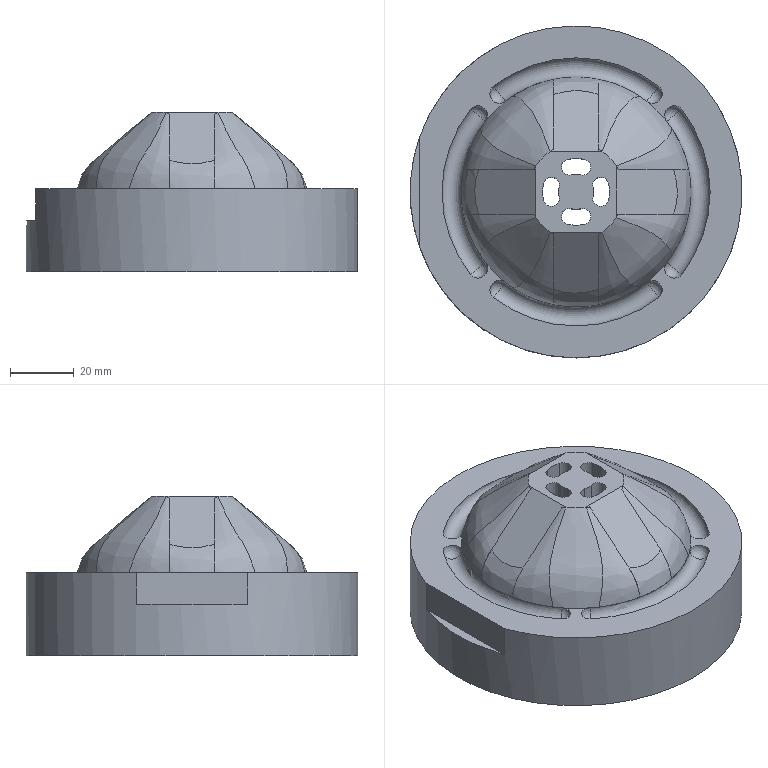NC program | NX | posted with a generic post | part box 104 x 104 x 49.86 mm
Lines 2861 to 4138 of 41131:
(PLANAR_MILL , TOOL : B)
N5714 M6
N5716 G54
N5718 G17 G0 G90 X-10.762 Y37.49 S2122 M3
N5720 G43 Z20. H0
N5722 Z-23.86
N5724 G94 G1 X-12.845 Y36.834 Z-23.87 F785.
N5726 X-15.067 Y35.983 Z-23.88
N5728 X-17.233 Y34.997 Z-23.891
N5730 X-19.335 Y33.881 Z-23.901
N5732 X-21.365 Y32.64 Z-23.911
N5734 X-23.315 Y31.276 Z-23.922
N5736 X-24.011 Y30.732 Z-23.926
N5738 X-23.315 Y31.276 Z-23.929
N5740 X-21.365 Y32.64 Z-23.94
N5742 X-19.335 Y33.881 Z-23.95
N5744 X-17.233 Y34.997 Z-23.961
N5746 X-15.067 Y35.983 Z-23.971
N5748 X-12.845 Y36.834 Z-23.981
N5750 X-10.576 Y37.549 Z-23.992
N5752 X-8.267 Y38.124 Z-24.002
N5754 X-5.927 Y38.557 Z-24.013
N5756 X-3.565 Y38.847 Z-24.023
N5758 X-1.19 Y38.992 Z-24.033
N5760 X1.19 Z-24.044
N5762 X3.565 Y38.847 Z-24.054
N5764 X5.927 Y38.557 Z-24.064
N5766 X8.267 Y38.124 Z-24.075
N5768 X10.576 Y37.549 Z-24.085
N5770 X12.845 Y36.834 Z-24.096
N5772 X15.067 Y35.983 Z-24.106
N5774 X17.233 Y34.997 Z-24.116
N5776 X19.335 Y33.881 Z-24.127
N5778 X21.365 Y32.64 Z-24.137
N5780 X23.315 Y31.276 Z-24.147
N5782 X24.011 Y30.732 Z-24.151
N5784 X23.315 Y31.276 Z-24.155
N5786 X21.365 Y32.64 Z-24.166
N5788 X19.335 Y33.881 Z-24.176
N5790 X17.233 Y34.997 Z-24.186
N5792 X15.067 Y35.983 Z-24.197
N5794 X12.845 Y36.834 Z-24.207
N5796 X10.576 Y37.549 Z-24.217
N5798 X8.267 Y38.124 Z-24.228
N5800 X5.927 Y38.557 Z-24.238
N5802 X3.565 Y38.847 Z-24.249
N5804 X1.19 Y38.992 Z-24.259
N5806 X-1.19 Z-24.269
N5808 X-3.565 Y38.847 Z-24.28
N5810 X-5.927 Y38.557 Z-24.29
N5812 X-8.267 Y38.124 Z-24.301
N5814 X-10.576 Y37.549 Z-24.311
N5816 X-12.845 Y36.834 Z-24.321
N5818 X-15.067 Y35.983 Z-24.332
N5820 X-17.233 Y34.997 Z-24.342
N5822 X-19.335 Y33.881 Z-24.352
N5824 X-21.365 Y32.64 Z-24.363
N5826 X-23.315 Y31.276 Z-24.373
N5828 X-24.011 Y30.732 Z-24.377
N5830 X-23.315 Y31.276 Z-24.381
N5832 X-21.365 Y32.64 Z-24.391
N5834 X-19.335 Y33.881 Z-24.402
N5836 X-17.233 Y34.997 Z-24.412
N5838 X-15.067 Y35.983 Z-24.422
N5840 X-12.845 Y36.834 Z-24.433
N5842 X-10.576 Y37.549 Z-24.443
N5844 X-8.267 Y38.124 Z-24.454
N5846 X-5.927 Y38.557 Z-24.464
N5848 X-3.565 Y38.847 Z-24.474
N5850 X-1.19 Y38.992 Z-24.485
N5852 X1.19 Z-24.495
N5854 X3.565 Y38.847 Z-24.506
N5856 X5.927 Y38.557 Z-24.516
N5858 X8.267 Y38.124 Z-24.526
N5860 X10.576 Y37.549 Z-24.537
N5862 X12.845 Y36.834 Z-24.547
N5864 X15.067 Y35.983 Z-24.557
N5866 X17.233 Y34.997 Z-24.568
N5868 X19.335 Y33.881 Z-24.578
N5870 X21.365 Y32.64 Z-24.589
N5872 X23.315 Y31.276 Z-24.599
N5874 X24.011 Y30.732 Z-24.603
N5876 X23.315 Y31.276 Z-24.607
N5878 X21.365 Y32.64 Z-24.617
N5880 X19.335 Y33.881 Z-24.627
N5882 X17.233 Y34.997 Z-24.638
N5884 X15.067 Y35.983 Z-24.648
N5886 X12.845 Y36.834 Z-24.659
N5888 X10.576 Y37.549 Z-24.669
N5890 X8.267 Y38.124 Z-24.679
N5892 X5.927 Y38.557 Z-24.69
N5894 X3.565 Y38.847 Z-24.7
N5896 X1.19 Y38.992 Z-24.711
N5898 X-1.19 Z-24.721
N5900 X-3.565 Y38.847 Z-24.731
N5902 X-5.927 Y38.557 Z-24.742
N5904 X-8.267 Y38.124 Z-24.752
N5906 X-10.576 Y37.549 Z-24.762
N5908 X-12.845 Y36.834 Z-24.773
N5910 X-15.067 Y35.983 Z-24.783
N5912 X-17.233 Y34.997 Z-24.794
N5914 X-19.335 Y33.881 Z-24.804
N5916 X-21.365 Y32.64 Z-24.814
N5918 X-23.315 Y31.276 Z-24.825
N5920 X-24.011 Y30.732 Z-24.829
N5922 X-23.315 Y31.276 Z-24.832
N5924 X-21.365 Y32.64 Z-24.843
N5926 X-19.335 Y33.881 Z-24.853
N5928 X-17.233 Y34.997 Z-24.864
N5930 X-15.067 Y35.983 Z-24.874
N5932 X-12.845 Y36.834 Z-24.884
N5934 X-10.576 Y37.549 Z-24.895
N5936 X-8.267 Y38.124 Z-24.905
N5938 X-5.927 Y38.557 Z-24.915
N5940 X-3.565 Y38.847 Z-24.926
N5942 X-1.19 Y38.992 Z-24.936
N5944 X1.19 Z-24.947
N5946 X3.565 Y38.847 Z-24.957
N5948 X5.927 Y38.557 Z-24.967
N5950 X8.267 Y38.124 Z-24.978
N5952 X10.576 Y37.549 Z-24.988
N5954 X12.845 Y36.834 Z-24.999
N5956 X15.067 Y35.983 Z-25.009
N5958 X17.233 Y34.997 Z-25.019
N5960 X19.335 Y33.881 Z-25.03
N5962 X21.365 Y32.64 Z-25.04
N5964 X23.315 Y31.276 Z-25.05
N5966 X24.011 Y30.732 Z-25.054
N5968 X23.315 Y31.276 Z-25.058
N5970 X21.365 Y32.64 Z-25.069
N5972 X19.335 Y33.881 Z-25.079
N5974 X17.233 Y34.997 Z-25.089
N5976 X15.067 Y35.983 Z-25.1
N5978 X12.845 Y36.834 Z-25.11
N5980 X10.576 Y37.549 Z-25.12
N5982 X8.267 Y38.124 Z-25.131
N5984 X5.927 Y38.557 Z-25.141
N5986 X3.565 Y38.847 Z-25.152
N5988 X1.19 Y38.992 Z-25.162
N5990 X-1.19 Z-25.172
N5992 X-3.565 Y38.847 Z-25.183
N5994 X-5.927 Y38.557 Z-25.193
N5996 X-8.267 Y38.124 Z-25.204
N5998 X-10.576 Y37.549 Z-25.214
N6000 X-12.845 Y36.834 Z-25.224
N6002 X-15.067 Y35.983 Z-25.235
N6004 X-17.233 Y34.997 Z-25.245
N6006 X-19.335 Y33.881 Z-25.255
N6008 X-21.365 Y32.64 Z-25.266
N6010 X-23.315 Y31.276 Z-25.276
N6012 X-24.011 Y30.732 Z-25.28
N6014 X-23.315 Y31.276 Z-25.284
N6016 X-21.365 Y32.64 Z-25.294
N6018 X-19.335 Y33.881 Z-25.305
N6020 X-17.233 Y34.997 Z-25.315
N6022 X-15.067 Y35.983 Z-25.325
N6024 X-12.845 Y36.834 Z-25.336
N6026 X-10.576 Y37.549 Z-25.346
N6028 X-8.267 Y38.124 Z-25.357
N6030 X-5.927 Y38.557 Z-25.367
N6032 X-3.565 Y38.847 Z-25.377
N6034 X-1.19 Y38.992 Z-25.388
N6036 X1.19 Z-25.398
N6038 X3.565 Y38.847 Z-25.409
N6040 X5.927 Y38.557 Z-25.419
N6042 X8.267 Y38.124 Z-25.429
N6044 X10.576 Y37.549 Z-25.44
N6046 X12.845 Y36.834 Z-25.45
N6048 X15.067 Y35.983 Z-25.46
N6050 X17.233 Y34.997 Z-25.471
N6052 X19.335 Y33.881 Z-25.481
N6054 X21.365 Y32.64 Z-25.492
N6056 X23.315 Y31.276 Z-25.502
N6058 X24.011 Y30.732 Z-25.506
N6060 X23.315 Y31.276 Z-25.51
N6062 X21.365 Y32.64 Z-25.52
N6064 X19.335 Y33.881 Z-25.53
N6066 X17.233 Y34.997 Z-25.541
N6068 X15.067 Y35.983 Z-25.551
N6070 X12.845 Y36.834 Z-25.562
N6072 X10.576 Y37.549 Z-25.572
N6074 X8.267 Y38.124 Z-25.582
N6076 X5.927 Y38.557 Z-25.593
N6078 X3.565 Y38.847 Z-25.603
N6080 X1.19 Y38.992 Z-25.614
N6082 X-1.19 Z-25.624
N6084 X-3.565 Y38.847 Z-25.634
N6086 X-5.927 Y38.557 Z-25.645
N6088 X-8.267 Y38.124 Z-25.655
N6090 X-10.576 Y37.549 Z-25.665
N6092 X-12.845 Y36.834 Z-25.676
N6094 X-15.067 Y35.983 Z-25.686
N6096 X-17.233 Y34.997 Z-25.697
N6098 X-19.335 Y33.881 Z-25.707
N6100 X-21.365 Y32.64 Z-25.717
N6102 X-23.315 Y31.276 Z-25.728
N6104 X-24.011 Y30.732 Z-25.732
N6106 X-23.315 Y31.276 Z-25.735
N6108 X-21.365 Y32.64 Z-25.746
N6110 X-19.335 Y33.881 Z-25.756
N6112 X-17.233 Y34.997 Z-25.767
N6114 X-15.067 Y35.983 Z-25.777
N6116 X-12.845 Y36.834 Z-25.787
N6118 X-10.576 Y37.549 Z-25.798
N6120 X-8.267 Y38.124 Z-25.808
N6122 X-5.927 Y38.557 Z-25.818
N6124 X-3.565 Y38.847 Z-25.829
N6126 X-1.19 Y38.992 Z-25.839
N6128 X1.19 Z-25.85
N6130 X3.565 Y38.847 Z-25.86
N6132 X5.927 Y38.557 Z-25.87
N6134 X8.267 Y38.124 Z-25.881
N6136 X10.576 Y37.549 Z-25.891
N6138 X12.845 Y36.834 Z-25.902
N6140 X15.067 Y35.983 Z-25.912
N6142 X17.233 Y34.997 Z-25.922
N6144 X19.335 Y33.881 Z-25.933
N6146 X21.365 Y32.64 Z-25.943
N6148 X23.315 Y31.276 Z-25.953
N6150 X24.011 Y30.732 Z-25.957
N6152 X23.315 Y31.276 Z-25.961
N6154 X21.365 Y32.64 Z-25.972
N6156 X19.335 Y33.881 Z-25.982
N6158 X17.233 Y34.997 Z-25.992
N6160 X15.067 Y35.983 Z-26.003
N6162 X12.845 Y36.834 Z-26.013
N6164 X10.576 Y37.549 Z-26.023
N6166 X8.267 Y38.124 Z-26.034
N6168 X5.927 Y38.557 Z-26.044
N6170 X3.565 Y38.847 Z-26.055
N6172 X1.19 Y38.992 Z-26.065
N6174 X-1.19 Z-26.075
N6176 X-3.565 Y38.847 Z-26.086
N6178 X-5.927 Y38.557 Z-26.096
N6180 X-8.267 Y38.124 Z-26.107
N6182 X-10.576 Y37.549 Z-26.117
N6184 X-12.845 Y36.834 Z-26.127
N6186 X-15.067 Y35.983 Z-26.138
N6188 X-17.233 Y34.997 Z-26.148
N6190 X-19.335 Y33.881 Z-26.158
N6192 X-21.365 Y32.64 Z-26.169
N6194 X-23.315 Y31.276 Z-26.179
N6196 X-24.011 Y30.732 Z-26.183
N6198 X-23.315 Y31.276 Z-26.187
N6200 X-21.365 Y32.64 Z-26.197
N6202 X-19.335 Y33.881 Z-26.208
N6204 X-17.233 Y34.997 Z-26.218
N6206 X-15.067 Y35.983 Z-26.228
N6208 X-12.845 Y36.834 Z-26.239
N6210 X-10.576 Y37.549 Z-26.249
N6212 X-8.267 Y38.124 Z-26.26
N6214 X-5.927 Y38.557 Z-26.27
N6216 X-3.565 Y38.847 Z-26.28
N6218 X-1.19 Y38.992 Z-26.291
N6220 X1.19 Z-26.301
N6222 X3.565 Y38.847 Z-26.312
N6224 X5.927 Y38.557 Z-26.322
N6226 X8.267 Y38.124 Z-26.332
N6228 X10.576 Y37.549 Z-26.343
N6230 X12.845 Y36.834 Z-26.353
N6232 X15.067 Y35.983 Z-26.363
N6234 X17.233 Y34.997 Z-26.374
N6236 X19.335 Y33.881 Z-26.384
N6238 X21.365 Y32.64 Z-26.395
N6240 X23.315 Y31.276 Z-26.405
N6242 X24.011 Y30.732 Z-26.409
N6244 X23.315 Y31.276 Z-26.413
N6246 X21.365 Y32.64 Z-26.423
N6248 X19.335 Y33.881 Z-26.433
N6250 X17.233 Y34.997 Z-26.444
N6252 X15.067 Y35.983 Z-26.454
N6254 X12.845 Y36.834 Z-26.465
N6256 X10.576 Y37.549 Z-26.475
N6258 X8.267 Y38.124 Z-26.485
N6260 X5.927 Y38.557 Z-26.496
N6262 X3.565 Y38.847 Z-26.506
N6264 X1.19 Y38.992 Z-26.516
N6266 X-1.19 Z-26.527
N6268 X-3.565 Y38.847 Z-26.537
N6270 X-5.927 Y38.557 Z-26.548
N6272 X-8.267 Y38.124 Z-26.558
N6274 X-10.576 Y37.549 Z-26.568
N6276 X-12.845 Y36.834 Z-26.579
N6278 X-15.067 Y35.983 Z-26.589
N6280 X-17.233 Y34.997 Z-26.6
N6282 X-19.335 Y33.881 Z-26.61
N6284 X-21.365 Y32.64 Z-26.62
N6286 X-23.315 Y31.276 Z-26.631
N6288 X-24.011 Y30.732 Z-26.635
N6290 X-23.315 Y31.276 Z-26.638
N6292 X-21.365 Y32.64 Z-26.649
N6294 X-19.335 Y33.881 Z-26.659
N6296 X-17.233 Y34.997 Z-26.67
N6298 X-15.067 Y35.983 Z-26.68
N6300 X-12.845 Y36.834 Z-26.69
N6302 X-10.576 Y37.549 Z-26.701
N6304 X-8.267 Y38.124 Z-26.711
N6306 X-5.927 Y38.557 Z-26.721
N6308 X-3.565 Y38.847 Z-26.732
N6310 X-1.19 Y38.992 Z-26.742
N6312 X1.19 Z-26.753
N6314 X3.565 Y38.847 Z-26.763
N6316 X5.927 Y38.557 Z-26.773
N6318 X8.267 Y38.124 Z-26.784
N6320 X10.576 Y37.549 Z-26.794
N6322 X12.845 Y36.834 Z-26.805
N6324 X15.067 Y35.983 Z-26.815
N6326 X17.233 Y34.997 Z-26.825
N6328 X19.335 Y33.881 Z-26.836
N6330 X21.365 Y32.64 Z-26.846
N6332 X23.315 Y31.276 Z-26.856
N6334 X24.011 Y30.732 Z-26.86
N6336 G3 X-24.011 Y30.732 R39.
N6338 G1 Z-23.86
N6340 G0 Z20.
N6342 X-37.49 Y-10.762
N6344 Z-23.86
N6346 G1 X-36.834 Y-12.845 Z-23.87
N6348 X-35.983 Y-15.067 Z-23.88
N6350 X-34.997 Y-17.233 Z-23.891
N6352 X-33.881 Y-19.335 Z-23.901
N6354 X-32.64 Y-21.365 Z-23.911
N6356 X-31.276 Y-23.315 Z-23.922
N6358 X-30.732 Y-24.011 Z-23.926
N6360 X-31.276 Y-23.315 Z-23.929
N6362 X-32.64 Y-21.365 Z-23.94
N6364 X-33.881 Y-19.335 Z-23.95
N6366 X-34.997 Y-17.233 Z-23.961
N6368 X-35.983 Y-15.067 Z-23.971
N6370 X-36.834 Y-12.845 Z-23.981
N6372 X-37.549 Y-10.576 Z-23.992
N6374 X-38.124 Y-8.267 Z-24.002
N6376 X-38.557 Y-5.927 Z-24.013
N6378 X-38.847 Y-3.565 Z-24.023
N6380 X-38.992 Y-1.19 Z-24.033
N6382 Y1.19 Z-24.044
N6384 X-38.847 Y3.565 Z-24.054
N6386 X-38.557 Y5.927 Z-24.064
N6388 X-38.124 Y8.267 Z-24.075
N6390 X-37.549 Y10.576 Z-24.085
N6392 X-36.834 Y12.845 Z-24.096
N6394 X-35.983 Y15.067 Z-24.106
N6396 X-34.997 Y17.233 Z-24.116
N6398 X-33.881 Y19.335 Z-24.127
N6400 X-32.64 Y21.365 Z-24.137
N6402 X-31.276 Y23.315 Z-24.147
N6404 X-30.732 Y24.011 Z-24.151
N6406 X-31.276 Y23.315 Z-24.155
N6408 X-32.64 Y21.365 Z-24.166
N6410 X-33.881 Y19.335 Z-24.176
N6412 X-34.997 Y17.233 Z-24.186
N6414 X-35.983 Y15.067 Z-24.197
N6416 X-36.834 Y12.845 Z-24.207
N6418 X-37.549 Y10.576 Z-24.217
N6420 X-38.124 Y8.267 Z-24.228
N6422 X-38.557 Y5.927 Z-24.238
N6424 X-38.847 Y3.565 Z-24.249
N6426 X-38.992 Y1.19 Z-24.259
N6428 Y-1.19 Z-24.269
N6430 X-38.847 Y-3.565 Z-24.28
N6432 X-38.557 Y-5.927 Z-24.29
N6434 X-38.124 Y-8.267 Z-24.301
N6436 X-37.549 Y-10.576 Z-24.311
N6438 X-36.834 Y-12.845 Z-24.321
N6440 X-35.983 Y-15.067 Z-24.332
N6442 X-34.997 Y-17.233 Z-24.342
N6444 X-33.881 Y-19.335 Z-24.352
N6446 X-32.64 Y-21.365 Z-24.363
N6448 X-31.276 Y-23.315 Z-24.373
N6450 X-30.732 Y-24.011 Z-24.377
N6452 X-31.276 Y-23.315 Z-24.381
N6454 X-32.64 Y-21.365 Z-24.391
N6456 X-33.881 Y-19.335 Z-24.402
N6458 X-34.997 Y-17.233 Z-24.412
N6460 X-35.983 Y-15.067 Z-24.422
N6462 X-36.834 Y-12.845 Z-24.433
N6464 X-37.549 Y-10.576 Z-24.443
N6466 X-38.124 Y-8.267 Z-24.454
N6468 X-38.557 Y-5.927 Z-24.464
N6470 X-38.847 Y-3.565 Z-24.474
N6472 X-38.992 Y-1.19 Z-24.485
N6474 Y1.19 Z-24.495
N6476 X-38.847 Y3.565 Z-24.506
N6478 X-38.557 Y5.927 Z-24.516
N6480 X-38.124 Y8.267 Z-24.526
N6482 X-37.549 Y10.576 Z-24.537
N6484 X-36.834 Y12.845 Z-24.547
N6486 X-35.983 Y15.067 Z-24.557
N6488 X-34.997 Y17.233 Z-24.568
N6490 X-33.881 Y19.335 Z-24.578
N6492 X-32.64 Y21.365 Z-24.589
N6494 X-31.276 Y23.315 Z-24.599
N6496 X-30.732 Y24.011 Z-24.603
N6498 X-31.276 Y23.315 Z-24.607
N6500 X-32.64 Y21.365 Z-24.617
N6502 X-33.881 Y19.335 Z-24.627
N6504 X-34.997 Y17.233 Z-24.638
N6506 X-35.983 Y15.067 Z-24.648
N6508 X-36.834 Y12.845 Z-24.659
N6510 X-37.549 Y10.576 Z-24.669
N6512 X-38.124 Y8.267 Z-24.679
N6514 X-38.557 Y5.927 Z-24.69
N6516 X-38.847 Y3.565 Z-24.7
N6518 X-38.992 Y1.19 Z-24.711
N6520 Y-1.19 Z-24.721
N6522 X-38.847 Y-3.565 Z-24.731
N6524 X-38.557 Y-5.927 Z-24.742
N6526 X-38.124 Y-8.267 Z-24.752
N6528 X-37.549 Y-10.576 Z-24.762
N6530 X-36.834 Y-12.845 Z-24.773
N6532 X-35.983 Y-15.067 Z-24.783
N6534 X-34.997 Y-17.233 Z-24.794
N6536 X-33.881 Y-19.335 Z-24.804
N6538 X-32.64 Y-21.365 Z-24.814
N6540 X-31.276 Y-23.315 Z-24.825
N6542 X-30.732 Y-24.011 Z-24.829
N6544 X-31.276 Y-23.315 Z-24.832
N6546 X-32.64 Y-21.365 Z-24.843
N6548 X-33.881 Y-19.335 Z-24.853
N6550 X-34.997 Y-17.233 Z-24.864
N6552 X-35.983 Y-15.067 Z-24.874
N6554 X-36.834 Y-12.845 Z-24.884
N6556 X-37.549 Y-10.576 Z-24.895
N6558 X-38.124 Y-8.267 Z-24.905
N6560 X-38.557 Y-5.927 Z-24.915
N6562 X-38.847 Y-3.565 Z-24.926
N6564 X-38.992 Y-1.19 Z-24.936
N6566 Y1.19 Z-24.947
N6568 X-38.847 Y3.565 Z-24.957
N6570 X-38.557 Y5.927 Z-24.967
N6572 X-38.124 Y8.267 Z-24.978
N6574 X-37.549 Y10.576 Z-24.988
N6576 X-36.834 Y12.845 Z-24.999
N6578 X-35.983 Y15.067 Z-25.009
N6580 X-34.997 Y17.233 Z-25.019
N6582 X-33.881 Y19.335 Z-25.03
N6584 X-32.64 Y21.365 Z-25.04
N6586 X-31.276 Y23.315 Z-25.05
N6588 X-30.732 Y24.011 Z-25.054
N6590 X-31.276 Y23.315 Z-25.058
N6592 X-32.64 Y21.365 Z-25.069
N6594 X-33.881 Y19.335 Z-25.079
N6596 X-34.997 Y17.233 Z-25.089
N6598 X-35.983 Y15.067 Z-25.1
N6600 X-36.834 Y12.845 Z-25.11
N6602 X-37.549 Y10.576 Z-25.12
N6604 X-38.124 Y8.267 Z-25.131
N6606 X-38.557 Y5.927 Z-25.141
N6608 X-38.847 Y3.565 Z-25.152
N6610 X-38.992 Y1.19 Z-25.162
N6612 Y-1.19 Z-25.172
N6614 X-38.847 Y-3.565 Z-25.183
N6616 X-38.557 Y-5.927 Z-25.193
N6618 X-38.124 Y-8.267 Z-25.204
N6620 X-37.549 Y-10.576 Z-25.214
N6622 X-36.834 Y-12.845 Z-25.224
N6624 X-35.983 Y-15.067 Z-25.235
N6626 X-34.997 Y-17.233 Z-25.245
N6628 X-33.881 Y-19.335 Z-25.255
N6630 X-32.64 Y-21.365 Z-25.266
N6632 X-31.276 Y-23.315 Z-25.276
N6634 X-30.732 Y-24.011 Z-25.28
N6636 X-31.276 Y-23.315 Z-25.284
N6638 X-32.64 Y-21.365 Z-25.294
N6640 X-33.881 Y-19.335 Z-25.305
N6642 X-34.997 Y-17.233 Z-25.315
N6644 X-35.983 Y-15.067 Z-25.325
N6646 X-36.834 Y-12.845 Z-25.336
N6648 X-37.549 Y-10.576 Z-25.346
N6650 X-38.124 Y-8.267 Z-25.357
N6652 X-38.557 Y-5.927 Z-25.367
N6654 X-38.847 Y-3.565 Z-25.377
N6656 X-38.992 Y-1.19 Z-25.388
N6658 Y1.19 Z-25.398
N6660 X-38.847 Y3.565 Z-25.409
N6662 X-38.557 Y5.927 Z-25.419
N6664 X-38.124 Y8.267 Z-25.429
N6666 X-37.549 Y10.576 Z-25.44
N6668 X-36.834 Y12.845 Z-25.45
N6670 X-35.983 Y15.067 Z-25.46
N6672 X-34.997 Y17.233 Z-25.471
N6674 X-33.881 Y19.335 Z-25.481
N6676 X-32.64 Y21.365 Z-25.492
N6678 X-31.276 Y23.315 Z-25.502
N6680 X-30.732 Y24.011 Z-25.506
N6682 X-31.276 Y23.315 Z-25.51
N6684 X-32.64 Y21.365 Z-25.52
N6686 X-33.881 Y19.335 Z-25.53
N6688 X-34.997 Y17.233 Z-25.541
N6690 X-35.983 Y15.067 Z-25.551
N6692 X-36.834 Y12.845 Z-25.562
N6694 X-37.549 Y10.576 Z-25.572
N6696 X-38.124 Y8.267 Z-25.582
N6698 X-38.557 Y5.927 Z-25.593
N6700 X-38.847 Y3.565 Z-25.603
N6702 X-38.992 Y1.19 Z-25.614
N6704 Y-1.19 Z-25.624
N6706 X-38.847 Y-3.565 Z-25.634
N6708 X-38.557 Y-5.927 Z-25.645
N6710 X-38.124 Y-8.267 Z-25.655
N6712 X-37.549 Y-10.576 Z-25.665
N6714 X-36.834 Y-12.845 Z-25.676
N6716 X-35.983 Y-15.067 Z-25.686
N6718 X-34.997 Y-17.233 Z-25.697
N6720 X-33.881 Y-19.335 Z-25.707
N6722 X-32.64 Y-21.365 Z-25.717
N6724 X-31.276 Y-23.315 Z-25.728
N6726 X-30.732 Y-24.011 Z-25.732
N6728 X-31.276 Y-23.315 Z-25.735
N6730 X-32.64 Y-21.365 Z-25.746
N6732 X-33.881 Y-19.335 Z-25.756
N6734 X-34.997 Y-17.233 Z-25.767
N6736 X-35.983 Y-15.067 Z-25.777
N6738 X-36.834 Y-12.845 Z-25.787
N6740 X-37.549 Y-10.576 Z-25.798
N6742 X-38.124 Y-8.267 Z-25.808
N6744 X-38.557 Y-5.927 Z-25.818
N6746 X-38.847 Y-3.565 Z-25.829
N6748 X-38.992 Y-1.19 Z-25.839
N6750 Y1.19 Z-25.85
N6752 X-38.847 Y3.565 Z-25.86
N6754 X-38.557 Y5.927 Z-25.87
N6756 X-38.124 Y8.267 Z-25.881
N6758 X-37.549 Y10.576 Z-25.891
N6760 X-36.834 Y12.845 Z-25.902
N6762 X-35.983 Y15.067 Z-25.912
N6764 X-34.997 Y17.233 Z-25.922
N6766 X-33.881 Y19.335 Z-25.933
N6768 X-32.64 Y21.365 Z-25.943
N6770 X-31.276 Y23.315 Z-25.953
N6772 X-30.732 Y24.011 Z-25.957
N6774 X-31.276 Y23.315 Z-25.961
N6776 X-32.64 Y21.365 Z-25.972
N6778 X-33.881 Y19.335 Z-25.982
N6780 X-34.997 Y17.233 Z-25.992
N6782 X-35.983 Y15.067 Z-26.003
N6784 X-36.834 Y12.845 Z-26.013
N6786 X-37.549 Y10.576 Z-26.023
N6788 X-38.124 Y8.267 Z-26.034
N6790 X-38.557 Y5.927 Z-26.044
N6792 X-38.847 Y3.565 Z-26.055
N6794 X-38.992 Y1.19 Z-26.065
N6796 Y-1.19 Z-26.075
N6798 X-38.847 Y-3.565 Z-26.086
N6800 X-38.557 Y-5.927 Z-26.096
N6802 X-38.124 Y-8.267 Z-26.107
N6804 X-37.549 Y-10.576 Z-26.117
N6806 X-36.834 Y-12.845 Z-26.127
N6808 X-35.983 Y-15.067 Z-26.138
N6810 X-34.997 Y-17.233 Z-26.148
N6812 X-33.881 Y-19.335 Z-26.158
N6814 X-32.64 Y-21.365 Z-26.169
N6816 X-31.276 Y-23.315 Z-26.179
N6818 X-30.732 Y-24.011 Z-26.183
N6820 X-31.276 Y-23.315 Z-26.187
N6822 X-32.64 Y-21.365 Z-26.197
N6824 X-33.881 Y-19.335 Z-26.208
N6826 X-34.997 Y-17.233 Z-26.218
N6828 X-35.983 Y-15.067 Z-26.228
N6830 X-36.834 Y-12.845 Z-26.239
N6832 X-37.549 Y-10.576 Z-26.249
N6834 X-38.124 Y-8.267 Z-26.26
N6836 X-38.557 Y-5.927 Z-26.27
N6838 X-38.847 Y-3.565 Z-26.28
N6840 X-38.992 Y-1.19 Z-26.291
N6842 Y1.19 Z-26.301
N6844 X-38.847 Y3.565 Z-26.312
N6846 X-38.557 Y5.927 Z-26.322
N6848 X-38.124 Y8.267 Z-26.332
N6850 X-37.549 Y10.576 Z-26.343
N6852 X-36.834 Y12.845 Z-26.353
N6854 X-35.983 Y15.067 Z-26.363
N6856 X-34.997 Y17.233 Z-26.374
N6858 X-33.881 Y19.335 Z-26.384
N6860 X-32.64 Y21.365 Z-26.395
N6862 X-31.276 Y23.315 Z-26.405
N6864 X-30.732 Y24.011 Z-26.409
N6866 X-31.276 Y23.315 Z-26.413
N6868 X-32.64 Y21.365 Z-26.423
N6870 X-33.881 Y19.335 Z-26.433
N6872 X-34.997 Y17.233 Z-26.444
N6874 X-35.983 Y15.067 Z-26.454
N6876 X-36.834 Y12.845 Z-26.465
N6878 X-37.549 Y10.576 Z-26.475
N6880 X-38.124 Y8.267 Z-26.485
N6882 X-38.557 Y5.927 Z-26.496
N6884 X-38.847 Y3.565 Z-26.506
N6886 X-38.992 Y1.19 Z-26.516
N6888 Y-1.19 Z-26.527
N6890 X-38.847 Y-3.565 Z-26.537
N6892 X-38.557 Y-5.927 Z-26.548
N6894 X-38.124 Y-8.267 Z-26.558
N6896 X-37.549 Y-10.576 Z-26.568
N6898 X-36.834 Y-12.845 Z-26.579
N6900 X-35.983 Y-15.067 Z-26.589
N6902 X-34.997 Y-17.233 Z-26.6
N6904 X-33.881 Y-19.335 Z-26.61
N6906 X-32.64 Y-21.365 Z-26.62
N6908 X-31.276 Y-23.315 Z-26.631
N6910 X-30.732 Y-24.011 Z-26.635
N6912 X-31.276 Y-23.315 Z-26.638
N6914 X-32.64 Y-21.365 Z-26.649
N6916 X-33.881 Y-19.335 Z-26.659
N6918 X-34.997 Y-17.233 Z-26.67
N6920 X-35.983 Y-15.067 Z-26.68
N6922 X-36.834 Y-12.845 Z-26.69
N6924 X-37.549 Y-10.576 Z-26.701
N6926 X-38.124 Y-8.267 Z-26.711
N6928 X-38.557 Y-5.927 Z-26.721
N6930 X-38.847 Y-3.565 Z-26.732
N6932 X-38.992 Y-1.19 Z-26.742
N6934 Y1.19 Z-26.753
N6936 X-38.847 Y3.565 Z-26.763
N6938 X-38.557 Y5.927 Z-26.773
N6940 X-38.124 Y8.267 Z-26.784
N6942 X-37.549 Y10.576 Z-26.794
N6944 X-36.834 Y12.845 Z-26.805
N6946 X-35.983 Y15.067 Z-26.815
N6948 X-34.997 Y17.233 Z-26.825
N6950 X-33.881 Y19.335 Z-26.836
N6952 X-32.64 Y21.365 Z-26.846
N6954 X-31.276 Y23.315 Z-26.856
N6956 X-30.732 Y24.011 Z-26.86
N6958 G3 X-30.732 Y-24.011 R39.
N6960 G1 Z-23.86
N6962 G0 Z20.
N6964 X10.762 Y-37.49
N6966 Z-23.86
N6968 G1 X12.845 Y-36.834 Z-23.87
N6970 X15.067 Y-35.983 Z-23.88
N6972 X17.233 Y-34.997 Z-23.891
N6974 X19.335 Y-33.881 Z-23.901
N6976 X21.365 Y-32.64 Z-23.911
N6978 X23.315 Y-31.276 Z-23.922
N6980 X24.011 Y-30.732 Z-23.926
N6982 X23.315 Y-31.276 Z-23.929
N6984 X21.365 Y-32.64 Z-23.94
N6986 X19.335 Y-33.881 Z-23.95
N6988 X17.233 Y-34.997 Z-23.961
N6990 X15.067 Y-35.983 Z-23.971
N6992 X12.845 Y-36.834 Z-23.981
N6994 X10.576 Y-37.549 Z-23.992
N6996 X8.267 Y-38.124 Z-24.002
N6998 X5.927 Y-38.557 Z-24.013
N7000 X3.565 Y-38.847 Z-24.023
N7002 X1.19 Y-38.992 Z-24.033
N7004 X-1.19 Z-24.044
N7006 X-3.565 Y-38.847 Z-24.054
N7008 X-5.927 Y-38.557 Z-24.064
N7010 X-8.267 Y-38.124 Z-24.075
N7012 X-10.576 Y-37.549 Z-24.085
N7014 X-12.845 Y-36.834 Z-24.096
N7016 X-15.067 Y-35.983 Z-24.106
N7018 X-17.233 Y-34.997 Z-24.116
N7020 X-19.335 Y-33.881 Z-24.127
N7022 X-21.365 Y-32.64 Z-24.137
N7024 X-23.315 Y-31.276 Z-24.147
N7026 X-24.011 Y-30.732 Z-24.151
N7028 X-23.315 Y-31.276 Z-24.155
N7030 X-21.365 Y-32.64 Z-24.166
N7032 X-19.335 Y-33.881 Z-24.176
N7034 X-17.233 Y-34.997 Z-24.186
N7036 X-15.067 Y-35.983 Z-24.197
N7038 X-12.845 Y-36.834 Z-24.207
N7040 X-10.576 Y-37.549 Z-24.217
N7042 X-8.267 Y-38.124 Z-24.228
N7044 X-5.927 Y-38.557 Z-24.238
N7046 X-3.565 Y-38.847 Z-24.249
N7048 X-1.19 Y-38.992 Z-24.259
N7050 X1.19 Z-24.269
N7052 X3.565 Y-38.847 Z-24.28
N7054 X5.927 Y-38.557 Z-24.29
N7056 X8.267 Y-38.124 Z-24.301
N7058 X10.576 Y-37.549 Z-24.311
N7060 X12.845 Y-36.834 Z-24.321
N7062 X15.067 Y-35.983 Z-24.332
N7064 X17.233 Y-34.997 Z-24.342
N7066 X19.335 Y-33.881 Z-24.352
N7068 X21.365 Y-32.64 Z-24.363
N7070 X23.315 Y-31.276 Z-24.373
N7072 X24.011 Y-30.732 Z-24.377
N7074 X23.315 Y-31.276 Z-24.381
N7076 X21.365 Y-32.64 Z-24.391
N7078 X19.335 Y-33.881 Z-24.402
N7080 X17.233 Y-34.997 Z-24.412
N7082 X15.067 Y-35.983 Z-24.422
N7084 X12.845 Y-36.834 Z-24.433
N7086 X10.576 Y-37.549 Z-24.443
N7088 X8.267 Y-38.124 Z-24.454
N7090 X5.927 Y-38.557 Z-24.464
N7092 X3.565 Y-38.847 Z-24.474
N7094 X1.19 Y-38.992 Z-24.485
N7096 X-1.19 Z-24.495
N7098 X-3.565 Y-38.847 Z-24.506
N7100 X-5.927 Y-38.557 Z-24.516
N7102 X-8.267 Y-38.124 Z-24.526
N7104 X-10.576 Y-37.549 Z-24.537
N7106 X-12.845 Y-36.834 Z-24.547
N7108 X-15.067 Y-35.983 Z-24.557
N7110 X-17.233 Y-34.997 Z-24.568
N7112 X-19.335 Y-33.881 Z-24.578
N7114 X-21.365 Y-32.64 Z-24.589
N7116 X-23.315 Y-31.276 Z-24.599
N7118 X-24.011 Y-30.732 Z-24.603
N7120 X-23.315 Y-31.276 Z-24.607
N7122 X-21.365 Y-32.64 Z-24.617
N7124 X-19.335 Y-33.881 Z-24.627
N7126 X-17.233 Y-34.997 Z-24.638
N7128 X-15.067 Y-35.983 Z-24.648
N7130 X-12.845 Y-36.834 Z-24.659
N7132 X-10.576 Y-37.549 Z-24.669
N7134 X-8.267 Y-38.124 Z-24.679
N7136 X-5.927 Y-38.557 Z-24.69
N7138 X-3.565 Y-38.847 Z-24.7
N7140 X-1.19 Y-38.992 Z-24.711
N7142 X1.19 Z-24.721
N7144 X3.565 Y-38.847 Z-24.731
N7146 X5.927 Y-38.557 Z-24.742
N7148 X8.267 Y-38.124 Z-24.752
N7150 X10.576 Y-37.549 Z-24.762
N7152 X12.845 Y-36.834 Z-24.773
N7154 X15.067 Y-35.983 Z-24.783
N7156 X17.233 Y-34.997 Z-24.794
N7158 X19.335 Y-33.881 Z-24.804
N7160 X21.365 Y-32.64 Z-24.814
N7162 X23.315 Y-31.276 Z-24.825
N7164 X24.011 Y-30.732 Z-24.829
N7166 X23.315 Y-31.276 Z-24.832
N7168 X21.365 Y-32.64 Z-24.843
N7170 X19.335 Y-33.881 Z-24.853
N7172 X17.233 Y-34.997 Z-24.864
N7174 X15.067 Y-35.983 Z-24.874
N7176 X12.845 Y-36.834 Z-24.884
N7178 X10.576 Y-37.549 Z-24.895
N7180 X8.267 Y-38.124 Z-24.905
N7182 X5.927 Y-38.557 Z-24.915
N7184 X3.565 Y-38.847 Z-24.926
N7186 X1.19 Y-38.992 Z-24.936
N7188 X-1.19 Z-24.947
N7190 X-3.565 Y-38.847 Z-24.957
N7192 X-5.927 Y-38.557 Z-24.967
N7194 X-8.267 Y-38.124 Z-24.978
N7196 X-10.576 Y-37.549 Z-24.988
N7198 X-12.845 Y-36.834 Z-24.999
N7200 X-15.067 Y-35.983 Z-25.009
N7202 X-17.233 Y-34.997 Z-25.019
N7204 X-19.335 Y-33.881 Z-25.03
N7206 X-21.365 Y-32.64 Z-25.04
N7208 X-23.315 Y-31.276 Z-25.05
N7210 X-24.011 Y-30.732 Z-25.054
N7212 X-23.315 Y-31.276 Z-25.058
N7214 X-21.365 Y-32.64 Z-25.069
N7216 X-19.335 Y-33.881 Z-25.079
N7218 X-17.233 Y-34.997 Z-25.089
N7220 X-15.067 Y-35.983 Z-25.1
N7222 X-12.845 Y-36.834 Z-25.11
N7224 X-10.576 Y-37.549 Z-25.12
N7226 X-8.267 Y-38.124 Z-25.131
N7228 X-5.927 Y-38.557 Z-25.141
N7230 X-3.565 Y-38.847 Z-25.152
N7232 X-1.19 Y-38.992 Z-25.162
N7234 X1.19 Z-25.172
N7236 X3.565 Y-38.847 Z-25.183
N7238 X5.927 Y-38.557 Z-25.193
N7240 X8.267 Y-38.124 Z-25.204
N7242 X10.576 Y-37.549 Z-25.214
N7244 X12.845 Y-36.834 Z-25.224
N7246 X15.067 Y-35.983 Z-25.235
N7248 X17.233 Y-34.997 Z-25.245
N7250 X19.335 Y-33.881 Z-25.255
N7252 X21.365 Y-32.64 Z-25.266
N7254 X23.315 Y-31.276 Z-25.276
N7256 X24.011 Y-30.732 Z-25.28
N7258 X23.315 Y-31.276 Z-25.284
N7260 X21.365 Y-32.64 Z-25.294
N7262 X19.335 Y-33.881 Z-25.305
N7264 X17.233 Y-34.997 Z-25.315
N7266 X15.067 Y-35.983 Z-25.325
N7268 X12.845 Y-36.834 Z-25.336
N7270 X10.576 Y-37.549 Z-25.346
N7272 X8.267 Y-38.124 Z-25.357
N7274 X5.927 Y-38.557 Z-25.367
N7276 X3.565 Y-38.847 Z-25.377
N7278 X1.19 Y-38.992 Z-25.388
N7280 X-1.19 Z-25.398
N7282 X-3.565 Y-38.847 Z-25.409
N7284 X-5.927 Y-38.557 Z-25.419
N7286 X-8.267 Y-38.124 Z-25.429
N7288 X-10.576 Y-37.549 Z-25.44
N7290 X-12.845 Y-36.834 Z-25.45
N7292 X-15.067 Y-35.983 Z-25.46
N7294 X-17.233 Y-34.997 Z-25.471
N7296 X-19.335 Y-33.881 Z-25.481
N7298 X-21.365 Y-32.64 Z-25.492
N7300 X-23.315 Y-31.276 Z-25.502
N7302 X-24.011 Y-30.732 Z-25.506
N7304 X-23.315 Y-31.276 Z-25.51
N7306 X-21.365 Y-32.64 Z-25.52
N7308 X-19.335 Y-33.881 Z-25.53
N7310 X-17.233 Y-34.997 Z-25.541
N7312 X-15.067 Y-35.983 Z-25.551
N7314 X-12.845 Y-36.834 Z-25.562
N7316 X-10.576 Y-37.549 Z-25.572
N7318 X-8.267 Y-38.124 Z-25.582
N7320 X-5.927 Y-38.557 Z-25.593
N7322 X-3.565 Y-38.847 Z-25.603
N7324 X-1.19 Y-38.992 Z-25.614
N7326 X1.19 Z-25.624
N7328 X3.565 Y-38.847 Z-25.634
N7330 X5.927 Y-38.557 Z-25.645
N7332 X8.267 Y-38.124 Z-25.655
N7334 X10.576 Y-37.549 Z-25.665
N7336 X12.845 Y-36.834 Z-25.676
N7338 X15.067 Y-35.983 Z-25.686
N7340 X17.233 Y-34.997 Z-25.697
N7342 X19.335 Y-33.881 Z-25.707
N7344 X21.365 Y-32.64 Z-25.717
N7346 X23.315 Y-31.276 Z-25.728
N7348 X24.011 Y-30.732 Z-25.732
N7350 X23.315 Y-31.276 Z-25.735
N7352 X21.365 Y-32.64 Z-25.746
N7354 X19.335 Y-33.881 Z-25.756
N7356 X17.233 Y-34.997 Z-25.767
N7358 X15.067 Y-35.983 Z-25.777
N7360 X12.845 Y-36.834 Z-25.787
N7362 X10.576 Y-37.549 Z-25.798
N7364 X8.267 Y-38.124 Z-25.808
N7366 X5.927 Y-38.557 Z-25.818
N7368 X3.565 Y-38.847 Z-25.829
N7370 X1.19 Y-38.992 Z-25.839
N7372 X-1.19 Z-25.85
N7374 X-3.565 Y-38.847 Z-25.86
N7376 X-5.927 Y-38.557 Z-25.87
N7378 X-8.267 Y-38.124 Z-25.881
N7380 X-10.576 Y-37.549 Z-25.891
N7382 X-12.845 Y-36.834 Z-25.902
N7384 X-15.067 Y-35.983 Z-25.912
N7386 X-17.233 Y-34.997 Z-25.922
N7388 X-19.335 Y-33.881 Z-25.933
N7390 X-21.365 Y-32.64 Z-25.943
N7392 X-23.315 Y-31.276 Z-25.953
N7394 X-24.011 Y-30.732 Z-25.957
N7396 X-23.315 Y-31.276 Z-25.961
N7398 X-21.365 Y-32.64 Z-25.972
N7400 X-19.335 Y-33.881 Z-25.982
N7402 X-17.233 Y-34.997 Z-25.992
N7404 X-15.067 Y-35.983 Z-26.003
N7406 X-12.845 Y-36.834 Z-26.013
N7408 X-10.576 Y-37.549 Z-26.023
N7410 X-8.267 Y-38.124 Z-26.034
N7412 X-5.927 Y-38.557 Z-26.044
N7414 X-3.565 Y-38.847 Z-26.055
N7416 X-1.19 Y-38.992 Z-26.065
N7418 X1.19 Z-26.075
N7420 X3.565 Y-38.847 Z-26.086
N7422 X5.927 Y-38.557 Z-26.096
N7424 X8.267 Y-38.124 Z-26.107
N7426 X10.576 Y-37.549 Z-26.117
N7428 X12.845 Y-36.834 Z-26.127
N7430 X15.067 Y-35.983 Z-26.138
N7432 X17.233 Y-34.997 Z-26.148
N7434 X19.335 Y-33.881 Z-26.158
N7436 X21.365 Y-32.64 Z-26.169
N7438 X23.315 Y-31.276 Z-26.179
N7440 X24.011 Y-30.732 Z-26.183
N7442 X23.315 Y-31.276 Z-26.187
N7444 X21.365 Y-32.64 Z-26.197
N7446 X19.335 Y-33.881 Z-26.208
N7448 X17.233 Y-34.997 Z-26.218
N7450 X15.067 Y-35.983 Z-26.228
N7452 X12.845 Y-36.834 Z-26.239
N7454 X10.576 Y-37.549 Z-26.249
N7456 X8.267 Y-38.124 Z-26.26
N7458 X5.927 Y-38.557 Z-26.27
N7460 X3.565 Y-38.847 Z-26.28
N7462 X1.19 Y-38.992 Z-26.291
N7464 X-1.19 Z-26.301
N7466 X-3.565 Y-38.847 Z-26.312
N7468 X-5.927 Y-38.557 Z-26.322
N7470 X-8.267 Y-38.124 Z-26.332
N7472 X-10.576 Y-37.549 Z-26.343
N7474 X-12.845 Y-36.834 Z-26.353
N7476 X-15.067 Y-35.983 Z-26.363
N7478 X-17.233 Y-34.997 Z-26.374
N7480 X-19.335 Y-33.881 Z-26.384
N7482 X-21.365 Y-32.64 Z-26.395
N7484 X-23.315 Y-31.276 Z-26.405
N7486 X-24.011 Y-30.732 Z-26.409
N7488 X-23.315 Y-31.276 Z-26.413
N7490 X-21.365 Y-32.64 Z-26.423
N7492 X-19.335 Y-33.881 Z-26.433
N7494 X-17.233 Y-34.997 Z-26.444
N7496 X-15.067 Y-35.983 Z-26.454
N7498 X-12.845 Y-36.834 Z-26.465
N7500 X-10.576 Y-37.549 Z-26.475
N7502 X-8.267 Y-38.124 Z-26.485
N7504 X-5.927 Y-38.557 Z-26.496
N7506 X-3.565 Y-38.847 Z-26.506
N7508 X-1.19 Y-38.992 Z-26.516
N7510 X1.19 Z-26.527
N7512 X3.565 Y-38.847 Z-26.537
N7514 X5.927 Y-38.557 Z-26.548
N7516 X8.267 Y-38.124 Z-26.558
N7518 X10.576 Y-37.549 Z-26.568
N7520 X12.845 Y-36.834 Z-26.579
N7522 X15.067 Y-35.983 Z-26.589
N7524 X17.233 Y-34.997 Z-26.6
N7526 X19.335 Y-33.881 Z-26.61
N7528 X21.365 Y-32.64 Z-26.62
N7530 X23.315 Y-31.276 Z-26.631
N7532 X24.011 Y-30.732 Z-26.635
N7534 X23.315 Y-31.276 Z-26.638
N7536 X21.365 Y-32.64 Z-26.649
N7538 X19.335 Y-33.881 Z-26.659
N7540 X17.233 Y-34.997 Z-26.67
N7542 X15.067 Y-35.983 Z-26.68
N7544 X12.845 Y-36.834 Z-26.69
N7546 X10.576 Y-37.549 Z-26.701
N7548 X8.267 Y-38.124 Z-26.711
N7550 X5.927 Y-38.557 Z-26.721
N7552 X3.565 Y-38.847 Z-26.732
N7554 X1.19 Y-38.992 Z-26.742
N7556 X-1.19 Z-26.753
N7558 X-3.565 Y-38.847 Z-26.763
N7560 X-5.927 Y-38.557 Z-26.773
N7562 X-8.267 Y-38.124 Z-26.784
N7564 X-10.576 Y-37.549 Z-26.794
N7566 X-12.845 Y-36.834 Z-26.805
N7568 X-15.067 Y-35.983 Z-26.815
N7570 X-17.233 Y-34.997 Z-26.825
N7572 X-19.335 Y-33.881 Z-26.836
N7574 X-21.365 Y-32.64 Z-26.846
N7576 X-23.315 Y-31.276 Z-26.856
N7578 X-24.011 Y-30.732 Z-26.86
N7580 G3 X24.011 Y-30.732 R39.
N7582 G1 Z-23.86
N7584 G0 Z20.
N7586 X37.49 Y10.762
N7588 Z-23.86
N7590 G1 X36.834 Y12.845 Z-23.87
N7592 X35.983 Y15.067 Z-23.88
N7594 X34.997 Y17.233 Z-23.891
N7596 X33.881 Y19.335 Z-23.901
N7598 X32.64 Y21.365 Z-23.911
N7600 X31.276 Y23.315 Z-23.922
N7602 X30.732 Y24.011 Z-23.926
N7604 X31.276 Y23.315 Z-23.929
N7606 X32.64 Y21.365 Z-23.94
N7608 X33.881 Y19.335 Z-23.95
N7610 X34.997 Y17.233 Z-23.961
N7612 X35.983 Y15.067 Z-23.971
N7614 X36.834 Y12.845 Z-23.981
N7616 X37.549 Y10.576 Z-23.992
N7618 X38.124 Y8.267 Z-24.002
N7620 X38.557 Y5.927 Z-24.013
N7622 X38.847 Y3.565 Z-24.023
N7624 X38.992 Y1.19 Z-24.033
N7626 Y-1.19 Z-24.044
N7628 X38.847 Y-3.565 Z-24.054
N7630 X38.557 Y-5.927 Z-24.064
N7632 X38.124 Y-8.267 Z-24.075
N7634 X37.549 Y-10.576 Z-24.085
N7636 X36.834 Y-12.845 Z-24.096
N7638 X35.983 Y-15.067 Z-24.106
N7640 X34.997 Y-17.233 Z-24.116
N7642 X33.881 Y-19.335 Z-24.127
N7644 X32.64 Y-21.365 Z-24.137
N7646 X31.276 Y-23.315 Z-24.147
N7648 X30.732 Y-24.011 Z-24.151
N7650 X31.276 Y-23.315 Z-24.155
N7652 X32.64 Y-21.365 Z-24.166
N7654 X33.881 Y-19.335 Z-24.176
N7656 X34.997 Y-17.233 Z-24.186
N7658 X35.983 Y-15.067 Z-24.197
N7660 X36.834 Y-12.845 Z-24.207
N7662 X37.549 Y-10.576 Z-24.217
N7664 X38.124 Y-8.267 Z-24.228
N7666 X38.557 Y-5.927 Z-24.238
N7668 X38.847 Y-3.565 Z-24.249
N7670 X38.992 Y-1.19 Z-24.259
N7672 Y1.19 Z-24.269
N7674 X38.847 Y3.565 Z-24.28
N7676 X38.557 Y5.927 Z-24.29
N7678 X38.124 Y8.267 Z-24.301
N7680 X37.549 Y10.576 Z-24.311
N7682 X36.834 Y12.845 Z-24.321
N7684 X35.983 Y15.067 Z-24.332
N7686 X34.997 Y17.233 Z-24.342
N7688 X33.881 Y19.335 Z-24.352
N7690 X32.64 Y21.365 Z-24.363
N7692 X31.276 Y23.315 Z-24.373
N7694 X30.732 Y24.011 Z-24.377
N7696 X31.276 Y23.315 Z-24.381
N7698 X32.64 Y21.365 Z-24.391
N7700 X33.881 Y19.335 Z-24.402
N7702 X34.997 Y17.233 Z-24.412
N7704 X35.983 Y15.067 Z-24.422
N7706 X36.834 Y12.845 Z-24.433
N7708 X37.549 Y10.576 Z-24.443
N7710 X38.124 Y8.267 Z-24.454
N7712 X38.557 Y5.927 Z-24.464
N7714 X38.847 Y3.565 Z-24.474
N7716 X38.992 Y1.19 Z-24.485
N7718 Y-1.19 Z-24.495
N7720 X38.847 Y-3.565 Z-24.506
N7722 X38.557 Y-5.927 Z-24.516
N7724 X38.124 Y-8.267 Z-24.526
N7726 X37.549 Y-10.576 Z-24.537
N7728 X36.834 Y-12.845 Z-24.547
N7730 X35.983 Y-15.067 Z-24.557
N7732 X34.997 Y-17.233 Z-24.568
N7734 X33.881 Y-19.335 Z-24.578
N7736 X32.64 Y-21.365 Z-24.589
N7738 X31.276 Y-23.315 Z-24.599
N7740 X30.732 Y-24.011 Z-24.603
N7742 X31.276 Y-23.315 Z-24.607
N7744 X32.64 Y-21.365 Z-24.617
N7746 X33.881 Y-19.335 Z-24.627
N7748 X34.997 Y-17.233 Z-24.638
N7750 X35.983 Y-15.067 Z-24.648
N7752 X36.834 Y-12.845 Z-24.659
N7754 X37.549 Y-10.576 Z-24.669
N7756 X38.124 Y-8.267 Z-24.679
N7758 X38.557 Y-5.927 Z-24.69
N7760 X38.847 Y-3.565 Z-24.7
N7762 X38.992 Y-1.19 Z-24.711
N7764 Y1.19 Z-24.721
N7766 X38.847 Y3.565 Z-24.731
N7768 X38.557 Y5.927 Z-24.742
N7770 X38.124 Y8.267 Z-24.752
N7772 X37.549 Y10.576 Z-24.762
N7774 X36.834 Y12.845 Z-24.773
N7776 X35.983 Y15.067 Z-24.783
N7778 X34.997 Y17.233 Z-24.794
N7780 X33.881 Y19.335 Z-24.804
N7782 X32.64 Y21.365 Z-24.814
N7784 X31.276 Y23.315 Z-24.825
N7786 X30.732 Y24.011 Z-24.829
N7788 X31.276 Y23.315 Z-24.832
N7790 X32.64 Y21.365 Z-24.843
N7792 X33.881 Y19.335 Z-24.853
N7794 X34.997 Y17.233 Z-24.864
N7796 X35.983 Y15.067 Z-24.874
N7798 X36.834 Y12.845 Z-24.884
N7800 X37.549 Y10.576 Z-24.895
N7802 X38.124 Y8.267 Z-24.905
N7804 X38.557 Y5.927 Z-24.915
N7806 X38.847 Y3.565 Z-24.926
N7808 X38.992 Y1.19 Z-24.936
N7810 Y-1.19 Z-24.947
N7812 X38.847 Y-3.565 Z-24.957
N7814 X38.557 Y-5.927 Z-24.967
N7816 X38.124 Y-8.267 Z-24.978
N7818 X37.549 Y-10.576 Z-24.988
N7820 X36.834 Y-12.845 Z-24.999
N7822 X35.983 Y-15.067 Z-25.009
N7824 X34.997 Y-17.233 Z-25.019
N7826 X33.881 Y-19.335 Z-25.03
N7828 X32.64 Y-21.365 Z-25.04
N7830 X31.276 Y-23.315 Z-25.05
N7832 X30.732 Y-24.011 Z-25.054
N7834 X31.276 Y-23.315 Z-25.058
N7836 X32.64 Y-21.365 Z-25.069
N7838 X33.881 Y-19.335 Z-25.079
N7840 X34.997 Y-17.233 Z-25.089
N7842 X35.983 Y-15.067 Z-25.1
N7844 X36.834 Y-12.845 Z-25.11
N7846 X37.549 Y-10.576 Z-25.12
N7848 X38.124 Y-8.267 Z-25.131
N7850 X38.557 Y-5.927 Z-25.141
N7852 X38.847 Y-3.565 Z-25.152
N7854 X38.992 Y-1.19 Z-25.162
N7856 Y1.19 Z-25.172
N7858 X38.847 Y3.565 Z-25.183
N7860 X38.557 Y5.927 Z-25.193
N7862 X38.124 Y8.267 Z-25.204
N7864 X37.549 Y10.576 Z-25.214
N7866 X36.834 Y12.845 Z-25.224
N7868 X35.983 Y15.067 Z-25.235
N7870 X34.997 Y17.233 Z-25.245
N7872 X33.881 Y19.335 Z-25.255
N7874 X32.64 Y21.365 Z-25.266
N7876 X31.276 Y23.315 Z-25.276
N7878 X30.732 Y24.011 Z-25.28
N7880 X31.276 Y23.315 Z-25.284
N7882 X32.64 Y21.365 Z-25.294
N7884 X33.881 Y19.335 Z-25.305
N7886 X34.997 Y17.233 Z-25.315
N7888 X35.983 Y15.067 Z-25.325
N7890 X36.834 Y12.845 Z-25.336
N7892 X37.549 Y10.576 Z-25.346
N7894 X38.124 Y8.267 Z-25.357
N7896 X38.557 Y5.927 Z-25.367
N7898 X38.847 Y3.565 Z-25.377
N7900 X38.992 Y1.19 Z-25.388
N7902 Y-1.19 Z-25.398
N7904 X38.847 Y-3.565 Z-25.409
N7906 X38.557 Y-5.927 Z-25.419
N7908 X38.124 Y-8.267 Z-25.429
N7910 X37.549 Y-10.576 Z-25.44
N7912 X36.834 Y-12.845 Z-25.45
N7914 X35.983 Y-15.067 Z-25.46
N7916 X34.997 Y-17.233 Z-25.471
N7918 X33.881 Y-19.335 Z-25.481
N7920 X32.64 Y-21.365 Z-25.492
N7922 X31.276 Y-23.315 Z-25.502
N7924 X30.732 Y-24.011 Z-25.506
N7926 X31.276 Y-23.315 Z-25.51
N7928 X32.64 Y-21.365 Z-25.52
N7930 X33.881 Y-19.335 Z-25.53
N7932 X34.997 Y-17.233 Z-25.541
N7934 X35.983 Y-15.067 Z-25.551
N7936 X36.834 Y-12.845 Z-25.562
N7938 X37.549 Y-10.576 Z-25.572
N7940 X38.124 Y-8.267 Z-25.582
N7942 X38.557 Y-5.927 Z-25.593
N7944 X38.847 Y-3.565 Z-25.603
N7946 X38.992 Y-1.19 Z-25.614
N7948 Y1.19 Z-25.624
N7950 X38.847 Y3.565 Z-25.634
N7952 X38.557 Y5.927 Z-25.645
N7954 X38.124 Y8.267 Z-25.655
N7956 X37.549 Y10.576 Z-25.665
N7958 X36.834 Y12.845 Z-25.676
N7960 X35.983 Y15.067 Z-25.686
N7962 X34.997 Y17.233 Z-25.697
N7964 X33.881 Y19.335 Z-25.707
N7966 X32.64 Y21.365 Z-25.717
N7968 X31.276 Y23.315 Z-25.728
N7970 X30.732 Y24.011 Z-25.732
N7972 X31.276 Y23.315 Z-25.735
N7974 X32.64 Y21.365 Z-25.746
N7976 X33.881 Y19.335 Z-25.756
N7978 X34.997 Y17.233 Z-25.767
N7980 X35.983 Y15.067 Z-25.777
N7982 X36.834 Y12.845 Z-25.787
N7984 X37.549 Y10.576 Z-25.798
N7986 X38.124 Y8.267 Z-25.808
N7988 X38.557 Y5.927 Z-25.818
N7990 X38.847 Y3.565 Z-25.829
N7992 X38.992 Y1.19 Z-25.839
N7994 Y-1.19 Z-25.85
N7996 X38.847 Y-3.565 Z-25.86
N7998 X38.557 Y-5.927 Z-25.87
N8000 X38.124 Y-8.267 Z-25.881
N8002 X37.549 Y-10.576 Z-25.891
N8004 X36.834 Y-12.845 Z-25.902
N8006 X35.983 Y-15.067 Z-25.912
N8008 X34.997 Y-17.233 Z-25.922
N8010 X33.881 Y-19.335 Z-25.933
N8012 X32.64 Y-21.365 Z-25.943
N8014 X31.276 Y-23.315 Z-25.953
N8016 X30.732 Y-24.011 Z-25.957
N8018 X31.276 Y-23.315 Z-25.961
N8020 X32.64 Y-21.365 Z-25.972
N8022 X33.881 Y-19.335 Z-25.982
N8024 X34.997 Y-17.233 Z-25.992
N8026 X35.983 Y-15.067 Z-26.003
N8028 X36.834 Y-12.845 Z-26.013
N8030 X37.549 Y-10.576 Z-26.023
N8032 X38.124 Y-8.267 Z-26.034
N8034 X38.557 Y-5.927 Z-26.044
N8036 X38.847 Y-3.565 Z-26.055
N8038 X38.992 Y-1.19 Z-26.065
N8040 Y1.19 Z-26.075
N8042 X38.847 Y3.565 Z-26.086
N8044 X38.557 Y5.927 Z-26.096
N8046 X38.124 Y8.267 Z-26.107
N8048 X37.549 Y10.576 Z-26.117
N8050 X36.834 Y12.845 Z-26.127
N8052 X35.983 Y15.067 Z-26.138
N8054 X34.997 Y17.233 Z-26.148
N8056 X33.881 Y19.335 Z-26.158
N8058 X32.64 Y21.365 Z-26.169
N8060 X31.276 Y23.315 Z-26.179
N8062 X30.732 Y24.011 Z-26.183
N8064 X31.276 Y23.315 Z-26.187
N8066 X32.64 Y21.365 Z-26.197
N8068 X33.881 Y19.335 Z-26.208
N8070 X34.997 Y17.233 Z-26.218
N8072 X35.983 Y15.067 Z-26.228
N8074 X36.834 Y12.845 Z-26.239
N8076 X37.549 Y10.576 Z-26.249
N8078 X38.124 Y8.267 Z-26.26
N8080 X38.557 Y5.927 Z-26.27
N8082 X38.847 Y3.565 Z-26.28
N8084 X38.992 Y1.19 Z-26.291
N8086 Y-1.19 Z-26.301
N8088 X38.847 Y-3.565 Z-26.312
N8090 X38.557 Y-5.927 Z-26.322
N8092 X38.124 Y-8.267 Z-26.332
N8094 X37.549 Y-10.576 Z-26.343
N8096 X36.834 Y-12.845 Z-26.353
N8098 X35.983 Y-15.067 Z-26.363
N8100 X34.997 Y-17.233 Z-26.374
N8102 X33.881 Y-19.335 Z-26.384
N8104 X32.64 Y-21.365 Z-26.395
N8106 X31.276 Y-23.315 Z-26.405
N8108 X30.732 Y-24.011 Z-26.409
N8110 X31.276 Y-23.315 Z-26.413
N8112 X32.64 Y-21.365 Z-26.423
N8114 X33.881 Y-19.335 Z-26.433
N8116 X34.997 Y-17.233 Z-26.444
N8118 X35.983 Y-15.067 Z-26.454
N8120 X36.834 Y-12.845 Z-26.465
N8122 X37.549 Y-10.576 Z-26.475
N8124 X38.124 Y-8.267 Z-26.485
N8126 X38.557 Y-5.927 Z-26.496
N8128 X38.847 Y-3.565 Z-26.506
N8130 X38.992 Y-1.19 Z-26.516
N8132 Y1.19 Z-26.527
N8134 X38.847 Y3.565 Z-26.537
N8136 X38.557 Y5.927 Z-26.548
N8138 X38.124 Y8.267 Z-26.558
N8140 X37.549 Y10.576 Z-26.568
N8142 X36.834 Y12.845 Z-26.579
N8144 X35.983 Y15.067 Z-26.589
N8146 X34.997 Y17.233 Z-26.6
N8148 X33.881 Y19.335 Z-26.61
N8150 X32.64 Y21.365 Z-26.62
N8152 X31.276 Y23.315 Z-26.631
N8154 X30.732 Y24.011 Z-26.635
N8156 X31.276 Y23.315 Z-26.638
N8158 X32.64 Y21.365 Z-26.649
N8160 X33.881 Y19.335 Z-26.659
N8162 X34.997 Y17.233 Z-26.67
N8164 X35.983 Y15.067 Z-26.68
N8166 X36.834 Y12.845 Z-26.69
N8168 X37.549 Y10.576 Z-26.701
N8170 X38.124 Y8.267 Z-26.711
N8172 X38.557 Y5.927 Z-26.721
N8174 X38.847 Y3.565 Z-26.732
N8176 X38.992 Y1.19 Z-26.742
N8178 Y-1.19 Z-26.753
N8180 X38.847 Y-3.565 Z-26.763
N8182 X38.557 Y-5.927 Z-26.773
N8184 X38.124 Y-8.267 Z-26.784
N8186 X37.549 Y-10.576 Z-26.794
N8188 X36.834 Y-12.845 Z-26.805
N8190 X35.983 Y-15.067 Z-26.815
N8192 X34.997 Y-17.233 Z-26.825
N8194 X33.881 Y-19.335 Z-26.836
N8196 X32.64 Y-21.365 Z-26.846
N8198 X31.276 Y-23.315 Z-26.856
N8200 X30.732 Y-24.011 Z-26.86
N8202 G3 X30.732 Y24.011 R39.
N8204 G1 Z-23.86
N8206 G0 Z20.
(PLANAR_MILL_COPY , TOOL : B)
N8208 X24.011 Y30.732
N8210 Z-23.86
N8212 G1 Z-26.86
N8214 G3 X-24.011 Y30.732 R39.
N8216 G1 Z-23.86
N8218 G0 Z20.
N8220 X-30.732 Y24.011
N8222 Z-23.86
N8224 G1 Z-26.86
N8226 G3 X-30.732 Y-24.011 R39.
N8228 G1 Z-23.86
N8230 G0 Z20.
N8232 X-24.011 Y-30.732
N8234 Z-23.86
N8236 G1 Z-26.86
N8238 G3 X24.011 Y-30.732 R39.
N8240 G1 Z-23.86
N8242 G0 Z20.
N8244 X30.732 Y-24.011
N8246 Z-23.86
N8248 G1 Z-26.86
N8250 G3 X30.732 Y24.011 R39.
N8252 G1 Z-23.86
N8254 G0 Z20.
N8256 M5